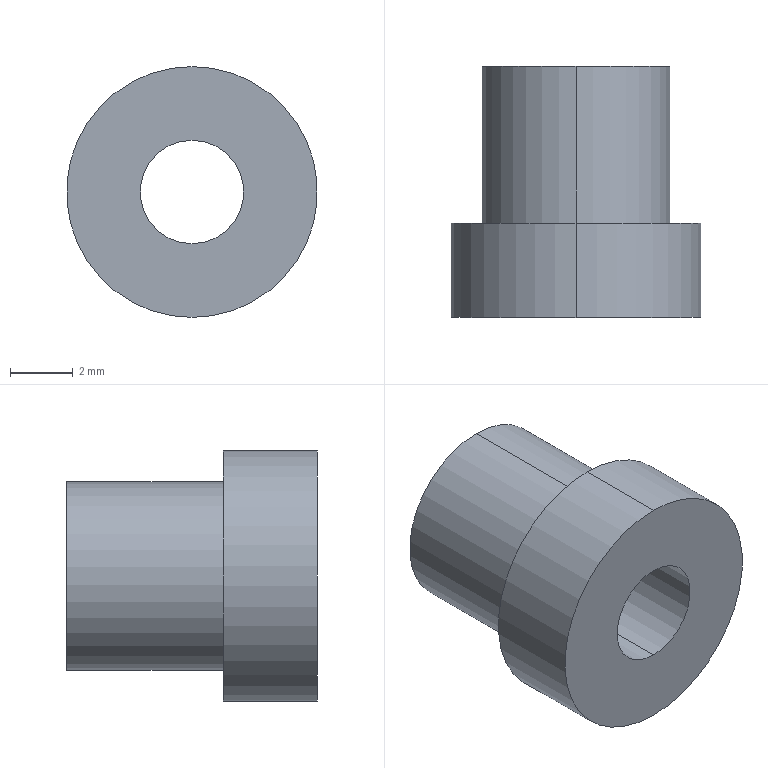Part | SolidWorks | features 3DProfileFeature 1, HoleWzd 1, Revolution 1 | 1 solid | 9 faces | box 8 x 8 x 8 mm | volume 223.744 mm3 | cylinder 6 | plane 3 | commonest cylinder face diameters 3.3 x2 6 x2 8 x2
STEP:
#1=CARTESIAN_POINT('',(0.,-8.,-1.65));
#2=VERTEX_POINT('',#1);
#3=CARTESIAN_POINT('',(0.,-8.,1.65));
#4=VERTEX_POINT('',#3);
#5=CARTESIAN_POINT('',(0.,-8.,0.));
#6=DIRECTION('',(0.,1.,0.));
#7=DIRECTION('',(0.,0.,1.));
#8=AXIS2_PLACEMENT_3D('',#5,#6,#7);
#9=CIRCLE('',#8,1.65);
#10=EDGE_CURVE('',#2,#4,#9,.T.);
#11=ORIENTED_EDGE('',*,*,#10,.F.);
#12=CARTESIAN_POINT('',(0.,0.,-1.65));
#13=VERTEX_POINT('',#12);
#14=CARTESIAN_POINT('',(0.,0.,-1.65));
#15=DIRECTION('',(0.,1.,0.));
#16=VECTOR('',#15,1000.);
#17=LINE('',#14,#16);
#18=EDGE_CURVE('',#2,#13,#17,.T.);
#19=ORIENTED_EDGE('',*,*,#18,.T.);
#20=CARTESIAN_POINT('',(0.,0.,1.65));
#21=VERTEX_POINT('',#20);
#22=CARTESIAN_POINT('',(0.,0.,0.));
#23=DIRECTION('',(0.,1.,0.));
#24=DIRECTION('',(0.,0.,1.));
#25=AXIS2_PLACEMENT_3D('',#22,#23,#24);
#26=CIRCLE('',#25,1.65);
#27=EDGE_CURVE('',#13,#21,#26,.T.);
#28=ORIENTED_EDGE('',*,*,#27,.T.);
#29=CARTESIAN_POINT('',(0.,0.,1.65));
#30=DIRECTION('',(0.,1.,0.));
#31=VECTOR('',#30,1000.);
#32=LINE('',#29,#31);
#33=EDGE_CURVE('',#4,#21,#32,.T.);
#34=ORIENTED_EDGE('',*,*,#33,.F.);
#35=EDGE_LOOP('',(#11,#19,#28,#34));
#36=FACE_OUTER_BOUND('',#35,.T.);
#37=CARTESIAN_POINT('',(0.,0.,0.));
#38=DIRECTION('',(0.,1.,0.));
#39=DIRECTION('',(0.,0.,1.));
#40=AXIS2_PLACEMENT_3D('',#37,#38,#39);
#41=CYLINDRICAL_SURFACE('',#40,1.65);
#42=ADVANCED_FACE('',(#36),#41,.F.);
#43=CARTESIAN_POINT('',(0.,-5.,3.));
#44=VERTEX_POINT('',#43);
#45=CARTESIAN_POINT('',(0.,-5.,-3.));
#46=VERTEX_POINT('',#45);
#47=CARTESIAN_POINT('',(0.,-5.,0.));
#48=DIRECTION('',(0.,1.,0.));
#49=DIRECTION('',(0.,0.,1.));
#50=AXIS2_PLACEMENT_3D('',#47,#48,#49);
#51=CIRCLE('',#50,3.);
#52=EDGE_CURVE('',#44,#46,#51,.T.);
#53=ORIENTED_EDGE('',*,*,#52,.T.);
#54=CARTESIAN_POINT('',(0.,0.,-3.));
#55=VERTEX_POINT('',#54);
#56=CARTESIAN_POINT('',(0.,0.,-3.));
#57=DIRECTION('',(0.,1.,0.));
#58=VECTOR('',#57,1000.);
#59=LINE('',#56,#58);
#60=EDGE_CURVE('',#46,#55,#59,.T.);
#61=ORIENTED_EDGE('',*,*,#60,.T.);
#62=CARTESIAN_POINT('',(0.,0.,3.));
#63=VERTEX_POINT('',#62);
#64=CARTESIAN_POINT('',(0.,0.,0.));
#65=DIRECTION('',(0.,1.,0.));
#66=DIRECTION('',(0.,0.,1.));
#67=AXIS2_PLACEMENT_3D('',#64,#65,#66);
#68=CIRCLE('',#67,3.);
#69=EDGE_CURVE('',#63,#55,#68,.T.);
#70=ORIENTED_EDGE('',*,*,#69,.F.);
#71=CARTESIAN_POINT('',(0.,0.,3.));
#72=DIRECTION('',(0.,1.,0.));
#73=VECTOR('',#72,1000.);
#74=LINE('',#71,#73);
#75=EDGE_CURVE('',#44,#63,#74,.T.);
#76=ORIENTED_EDGE('',*,*,#75,.F.);
#77=EDGE_LOOP('',(#53,#61,#70,#76));
#78=FACE_OUTER_BOUND('',#77,.T.);
#79=CARTESIAN_POINT('',(0.,0.,0.));
#80=DIRECTION('',(0.,1.,0.));
#81=DIRECTION('',(0.,0.,1.));
#82=AXIS2_PLACEMENT_3D('',#79,#80,#81);
#83=CYLINDRICAL_SURFACE('',#82,3.);
#84=ADVANCED_FACE('',(#78),#83,.T.);
#85=CARTESIAN_POINT('',(0.,-8.,4.));
#86=VERTEX_POINT('',#85);
#87=CARTESIAN_POINT('',(0.,-8.,-4.));
#88=VERTEX_POINT('',#87);
#89=CARTESIAN_POINT('',(0.,-8.,0.));
#90=DIRECTION('',(0.,1.,0.));
#91=DIRECTION('',(0.,0.,1.));
#92=AXIS2_PLACEMENT_3D('',#89,#90,#91);
#93=CIRCLE('',#92,4.);
#94=EDGE_CURVE('',#86,#88,#93,.T.);
#95=ORIENTED_EDGE('',*,*,#94,.T.);
#96=CARTESIAN_POINT('',(0.,-5.,-4.));
#97=VERTEX_POINT('',#96);
#98=CARTESIAN_POINT('',(0.,0.,-4.));
#99=DIRECTION('',(0.,1.,0.));
#100=VECTOR('',#99,1000.);
#101=LINE('',#98,#100);
#102=EDGE_CURVE('',#88,#97,#101,.T.);
#103=ORIENTED_EDGE('',*,*,#102,.T.);
#104=CARTESIAN_POINT('',(0.,-5.,4.));
#105=VERTEX_POINT('',#104);
#106=CARTESIAN_POINT('',(0.,-5.,0.));
#107=DIRECTION('',(0.,1.,0.));
#108=DIRECTION('',(0.,0.,1.));
#109=AXIS2_PLACEMENT_3D('',#106,#107,#108);
#110=CIRCLE('',#109,4.);
#111=EDGE_CURVE('',#105,#97,#110,.T.);
#112=ORIENTED_EDGE('',*,*,#111,.F.);
#113=CARTESIAN_POINT('',(0.,0.,4.));
#114=DIRECTION('',(0.,1.,0.));
#115=VECTOR('',#114,1000.);
#116=LINE('',#113,#115);
#117=EDGE_CURVE('',#86,#105,#116,.T.);
#118=ORIENTED_EDGE('',*,*,#117,.F.);
#119=EDGE_LOOP('',(#95,#103,#112,#118));
#120=FACE_OUTER_BOUND('',#119,.T.);
#121=CARTESIAN_POINT('',(0.,0.,0.));
#122=DIRECTION('',(0.,1.,0.));
#123=DIRECTION('',(0.,0.,1.));
#124=AXIS2_PLACEMENT_3D('',#121,#122,#123);
#125=CYLINDRICAL_SURFACE('',#124,4.);
#126=ADVANCED_FACE('',(#120),#125,.T.);
#127=CARTESIAN_POINT('',(0.,-8.,0.));
#128=DIRECTION('',(0.,1.,0.));
#129=DIRECTION('',(0.,0.,1.));
#130=AXIS2_PLACEMENT_3D('',#127,#128,#129);
#131=CIRCLE('',#130,1.65);
#132=EDGE_CURVE('',#4,#2,#131,.T.);
#133=ORIENTED_EDGE('',*,*,#132,.T.);
#134=ORIENTED_EDGE('',*,*,#10,.T.);
#135=EDGE_LOOP('',(#133,#134));
#136=FACE_BOUND('',#135,.T.);
#137=ORIENTED_EDGE('',*,*,#94,.F.);
#138=CARTESIAN_POINT('',(0.,-8.,0.));
#139=DIRECTION('',(0.,1.,0.));
#140=DIRECTION('',(0.,0.,1.));
#141=AXIS2_PLACEMENT_3D('',#138,#139,#140);
#142=CIRCLE('',#141,4.);
#143=EDGE_CURVE('',#88,#86,#142,.T.);
#144=ORIENTED_EDGE('',*,*,#143,.F.);
#145=EDGE_LOOP('',(#137,#144));
#146=FACE_OUTER_BOUND('',#145,.T.);
#147=CARTESIAN_POINT('',(0.,-8.,0.));
#148=DIRECTION('',(0.,1.,0.));
#149=DIRECTION('',(0.,0.,1.));
#150=AXIS2_PLACEMENT_3D('',#147,#148,#149);
#151=PLANE('',#150);
#152=ADVANCED_FACE('',(#136,#146),#151,.F.);
#153=ORIENTED_EDGE('',*,*,#102,.F.);
#154=ORIENTED_EDGE('',*,*,#143,.T.);
#155=ORIENTED_EDGE('',*,*,#117,.T.);
#156=CARTESIAN_POINT('',(0.,-5.,0.));
#157=DIRECTION('',(0.,1.,0.));
#158=DIRECTION('',(0.,0.,1.));
#159=AXIS2_PLACEMENT_3D('',#156,#157,#158);
#160=CIRCLE('',#159,4.);
#161=EDGE_CURVE('',#97,#105,#160,.T.);
#162=ORIENTED_EDGE('',*,*,#161,.F.);
#163=EDGE_LOOP('',(#153,#154,#155,#162));
#164=FACE_OUTER_BOUND('',#163,.T.);
#165=CARTESIAN_POINT('',(0.,0.,0.));
#166=DIRECTION('',(0.,1.,0.));
#167=DIRECTION('',(0.,0.,1.));
#168=AXIS2_PLACEMENT_3D('',#165,#166,#167);
#169=CYLINDRICAL_SURFACE('',#168,4.);
#170=ADVANCED_FACE('',(#164),#169,.T.);
#171=ORIENTED_EDGE('',*,*,#52,.F.);
#172=CARTESIAN_POINT('',(0.,-5.,0.));
#173=DIRECTION('',(0.,1.,0.));
#174=DIRECTION('',(0.,0.,1.));
#175=AXIS2_PLACEMENT_3D('',#172,#173,#174);
#176=CIRCLE('',#175,3.);
#177=EDGE_CURVE('',#46,#44,#176,.T.);
#178=ORIENTED_EDGE('',*,*,#177,.F.);
#179=EDGE_LOOP('',(#171,#178));
#180=FACE_BOUND('',#179,.T.);
#181=ORIENTED_EDGE('',*,*,#111,.T.);
#182=ORIENTED_EDGE('',*,*,#161,.T.);
#183=EDGE_LOOP('',(#181,#182));
#184=FACE_OUTER_BOUND('',#183,.T.);
#185=CARTESIAN_POINT('',(3.,-5.,0.));
#186=DIRECTION('',(0.,-1.,0.));
#187=DIRECTION('',(0.,0.,-1.));
#188=AXIS2_PLACEMENT_3D('',#185,#186,#187);
#189=PLANE('',#188);
#190=ADVANCED_FACE('',(#180,#184),#189,.F.);
#191=ORIENTED_EDGE('',*,*,#60,.F.);
#192=ORIENTED_EDGE('',*,*,#177,.T.);
#193=ORIENTED_EDGE('',*,*,#75,.T.);
#194=CARTESIAN_POINT('',(0.,0.,0.));
#195=DIRECTION('',(0.,1.,0.));
#196=DIRECTION('',(0.,0.,1.));
#197=AXIS2_PLACEMENT_3D('',#194,#195,#196);
#198=CIRCLE('',#197,3.);
#199=EDGE_CURVE('',#55,#63,#198,.T.);
#200=ORIENTED_EDGE('',*,*,#199,.F.);
#201=EDGE_LOOP('',(#191,#192,#193,#200));
#202=FACE_OUTER_BOUND('',#201,.T.);
#203=CARTESIAN_POINT('',(0.,0.,0.));
#204=DIRECTION('',(0.,1.,0.));
#205=DIRECTION('',(0.,0.,1.));
#206=AXIS2_PLACEMENT_3D('',#203,#204,#205);
#207=CYLINDRICAL_SURFACE('',#206,3.);
#208=ADVANCED_FACE('',(#202),#207,.T.);
#209=CARTESIAN_POINT('',(0.,0.,0.));
#210=DIRECTION('',(0.,1.,0.));
#211=DIRECTION('',(0.,0.,1.));
#212=AXIS2_PLACEMENT_3D('',#209,#210,#211);
#213=CIRCLE('',#212,1.65);
#214=EDGE_CURVE('',#21,#13,#213,.T.);
#215=ORIENTED_EDGE('',*,*,#214,.F.);
#216=ORIENTED_EDGE('',*,*,#27,.F.);
#217=EDGE_LOOP('',(#215,#216));
#218=FACE_BOUND('',#217,.T.);
#219=ORIENTED_EDGE('',*,*,#69,.T.);
#220=ORIENTED_EDGE('',*,*,#199,.T.);
#221=EDGE_LOOP('',(#219,#220));
#222=FACE_OUTER_BOUND('',#221,.T.);
#223=CARTESIAN_POINT('',(0.,0.,0.));
#224=DIRECTION('',(0.,-1.,0.));
#225=DIRECTION('',(0.,0.,-1.));
#226=AXIS2_PLACEMENT_3D('',#223,#224,#225);
#227=PLANE('',#226);
#228=ADVANCED_FACE('',(#218,#222),#227,.F.);
#229=ORIENTED_EDGE('',*,*,#18,.F.);
#230=ORIENTED_EDGE('',*,*,#132,.F.);
#231=ORIENTED_EDGE('',*,*,#33,.T.);
#232=ORIENTED_EDGE('',*,*,#214,.T.);
#233=EDGE_LOOP('',(#229,#230,#231,#232));
#234=FACE_OUTER_BOUND('',#233,.T.);
#235=CARTESIAN_POINT('',(0.,0.,0.));
#236=DIRECTION('',(0.,1.,0.));
#237=DIRECTION('',(0.,0.,1.));
#238=AXIS2_PLACEMENT_3D('',#235,#236,#237);
#239=CYLINDRICAL_SURFACE('',#238,1.65);
#240=ADVANCED_FACE('',(#234),#239,.F.);
#241=CLOSED_SHELL('',(#42,#84,#126,#152,#170,#190,#208,#228,#240));
#242=MANIFOLD_SOLID_BREP('',#241);
#243=CARTESIAN_POINT('',(0.,0.,0.));
#244=DIRECTION('',(0.,0.,1.));
#245=DIRECTION('',(1.,0.,0.));
#246=AXIS2_PLACEMENT_3D('',#243,#244,#245);
#247=(LENGTH_UNIT()NAMED_UNIT(*)SI_UNIT(.MILLI.,.METRE.));
#248=UNCERTAINTY_MEASURE_WITH_UNIT(LENGTH_MEASURE(0.00001),#247,'','');
#249=(NAMED_UNIT(*)PLANE_ANGLE_UNIT()SI_UNIT($,.RADIAN.));
#250=(NAMED_UNIT(*)SI_UNIT($,.STERADIAN.)SOLID_ANGLE_UNIT());
#251=(GEOMETRIC_REPRESENTATION_CONTEXT(3)GLOBAL_UNCERTAINTY_ASSIGNED_CONTEXT((#248))GLOBAL_UNIT_ASSIGNED_CONTEXT((#247,#249,#250))REPRESENTATION_CONTEXT('',''));
#252=ADVANCED_BREP_SHAPE_REPRESENTATION('',(#242,#246),#251);